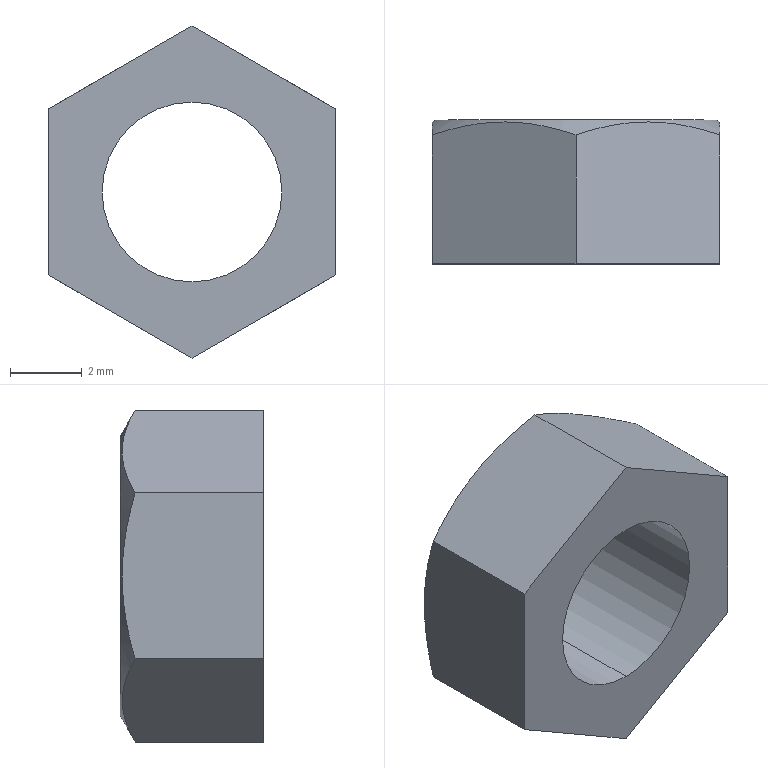Part | STEP file | NN19-M5 | 1 solid | 12 faces | box 8 x 4 x 9.238 mm | volume 142.232 mm3 | plane 8 | cylinder 2 | cone 2 | commonest cylinder face diameters 5 x2
STEP:
#1=CARTESIAN_POINT('',(0.,0.,0.));
#2=DIRECTION('',(0.,0.,1.));
#3=DIRECTION('',(1.,0.,0.));
#4=AXIS2_PLACEMENT_3D('',#1,#2,#3);
#5=CARTESIAN_POINT('',(0.,4.,-2.5));
#6=VERTEX_POINT('',#5);
#7=CARTESIAN_POINT('',(0.,0.,-2.5));
#8=VERTEX_POINT('',#7);
#9=CARTESIAN_POINT('',(0.,4.,-2.5));
#10=DIRECTION('',(0.,-1.,0.));
#11=VECTOR('',#10,1.);
#12=LINE('',#9,#11);
#13=CARTESIAN_POINT('',(0.,4.,0.));
#14=DIRECTION('',(0.,-1.,0.));
#15=DIRECTION('',(0.,0.,-1.));
#16=AXIS2_PLACEMENT_3D('',#13,#14,#15);
#17=CYLINDRICAL_SURFACE('',#16,2.5);
#18=CARTESIAN_POINT('',(6.283,0.));
#19=DIRECTION('',(0.,1.));
#20=VECTOR('',#19,1.);
#21=LINE('',#18,#20);
#22=(GEOMETRIC_REPRESENTATION_CONTEXT(2)PARAMETRIC_REPRESENTATION_CONTEXT()REPRESENTATION_CONTEXT('',''));
#23=DEFINITIONAL_REPRESENTATION('',(#21),#22);
#24=PCURVE('',#17,#23);
#25=CARTESIAN_POINT('',(0.,4.,0.));
#26=DIRECTION('',(0.,-1.,0.));
#27=DIRECTION('',(0.,0.,-1.));
#28=AXIS2_PLACEMENT_3D('',#25,#26,#27);
#29=CYLINDRICAL_SURFACE('',#28,2.5);
#30=CARTESIAN_POINT('',(0.,0.));
#31=DIRECTION('',(0.,1.));
#32=VECTOR('',#31,1.);
#33=LINE('',#30,#32);
#34=(GEOMETRIC_REPRESENTATION_CONTEXT(2)PARAMETRIC_REPRESENTATION_CONTEXT()REPRESENTATION_CONTEXT('',''));
#35=DEFINITIONAL_REPRESENTATION('',(#33),#34);
#36=PCURVE('',#29,#35);
#37=SURFACE_CURVE('',#12,(#24,#36),.PCURVE_S1.);
#38=EDGE_CURVE('',#6,#8,#37,.T.);
#39=ORIENTED_EDGE('',*,*,#38,.T.);
#40=CARTESIAN_POINT('',(0.,0.,2.5));
#41=VERTEX_POINT('',#40);
#42=CARTESIAN_POINT('',(0.,0.,0.));
#43=DIRECTION('',(0.,1.,0.));
#44=DIRECTION('',(0.,0.,1.));
#45=AXIS2_PLACEMENT_3D('',#42,#43,#44);
#46=CIRCLE('',#45,2.5);
#47=CARTESIAN_POINT('',(9.425,4.));
#48=DIRECTION('',(-1.,0.));
#49=VECTOR('',#48,1.);
#50=LINE('',#47,#49);
#51=(GEOMETRIC_REPRESENTATION_CONTEXT(2)PARAMETRIC_REPRESENTATION_CONTEXT()REPRESENTATION_CONTEXT('',''));
#52=DEFINITIONAL_REPRESENTATION('',(#50),#51);
#53=PCURVE('',#17,#52);
#54=CARTESIAN_POINT('',(0.,0.,0.));
#55=DIRECTION('',(0.,-1.,0.));
#56=DIRECTION('',(0.,0.,1.));
#57=AXIS2_PLACEMENT_3D('',#54,#55,#56);
#58=PLANE('',#57);
#59=CARTESIAN_POINT('',(2.5,0.));
#60=CARTESIAN_POINT('',(2.5,-4.33));
#61=CARTESIAN_POINT('',(-1.25,-2.165));
#62=CARTESIAN_POINT('',(-5.,0.));
#63=CARTESIAN_POINT('',(-1.25,2.165));
#64=CARTESIAN_POINT('',(2.5,4.33));
#65=CARTESIAN_POINT('',(2.5,0.));
#66=(BOUNDED_CURVE()B_SPLINE_CURVE(2,(#59,#60,#61,#62,#63,#64,#65),.UNSPECIFIED.,.T.,.F.)B_SPLINE_CURVE_WITH_KNOTS((1,2,2,2,2,1),(-2.094,0.,2.094,4.189,6.283,8.378),.UNSPECIFIED.)CURVE()GEOMETRIC_REPRESENTATION_ITEM()RATIONAL_B_SPLINE_CURVE((1.,0.5,1.,0.5,1.,0.5,1.))REPRESENTATION_ITEM(''));
#67=(GEOMETRIC_REPRESENTATION_CONTEXT(2)PARAMETRIC_REPRESENTATION_CONTEXT()REPRESENTATION_CONTEXT('',''));
#68=DEFINITIONAL_REPRESENTATION('',(#66),#67);
#69=PCURVE('',#58,#68);
#70=SURFACE_CURVE('',#46,(#53,#69),.PCURVE_S1.);
#71=EDGE_CURVE('',#8,#41,#70,.T.);
#72=ORIENTED_EDGE('',*,*,#71,.T.);
#73=CARTESIAN_POINT('',(0.,4.,2.5));
#74=VERTEX_POINT('',#73);
#75=CARTESIAN_POINT('',(0.,4.,2.5));
#76=DIRECTION('',(0.,-1.,0.));
#77=VECTOR('',#76,1.);
#78=LINE('',#75,#77);
#79=CARTESIAN_POINT('',(3.142,0.));
#80=DIRECTION('',(0.,1.));
#81=VECTOR('',#80,1.);
#82=LINE('',#79,#81);
#83=(GEOMETRIC_REPRESENTATION_CONTEXT(2)PARAMETRIC_REPRESENTATION_CONTEXT()REPRESENTATION_CONTEXT('',''));
#84=DEFINITIONAL_REPRESENTATION('',(#82),#83);
#85=PCURVE('',#17,#84);
#86=CARTESIAN_POINT('',(3.142,0.));
#87=DIRECTION('',(0.,1.));
#88=VECTOR('',#87,1.);
#89=LINE('',#86,#88);
#90=(GEOMETRIC_REPRESENTATION_CONTEXT(2)PARAMETRIC_REPRESENTATION_CONTEXT()REPRESENTATION_CONTEXT('',''));
#91=DEFINITIONAL_REPRESENTATION('',(#89),#90);
#92=PCURVE('',#29,#91);
#93=SURFACE_CURVE('',#78,(#85,#92),.PCURVE_S1.);
#94=EDGE_CURVE('',#74,#41,#93,.T.);
#95=ORIENTED_EDGE('',*,*,#94,.F.);
#96=CARTESIAN_POINT('',(0.,4.,0.));
#97=DIRECTION('',(0.,-1.,0.));
#98=DIRECTION('',(0.,0.,-1.));
#99=AXIS2_PLACEMENT_3D('',#96,#97,#98);
#100=CIRCLE('',#99,2.5);
#101=CARTESIAN_POINT('',(0.,0.));
#102=DIRECTION('',(1.,0.));
#103=VECTOR('',#102,1.);
#104=LINE('',#101,#103);
#105=(GEOMETRIC_REPRESENTATION_CONTEXT(2)PARAMETRIC_REPRESENTATION_CONTEXT()REPRESENTATION_CONTEXT('',''));
#106=DEFINITIONAL_REPRESENTATION('',(#104),#105);
#107=PCURVE('',#17,#106);
#108=CARTESIAN_POINT('',(0.,4.,0.));
#109=DIRECTION('',(0.,1.,0.));
#110=DIRECTION('',(-1.,0.,0.));
#111=AXIS2_PLACEMENT_3D('',#108,#109,#110);
#112=PLANE('',#111);
#113=CARTESIAN_POINT('',(0.,-2.5));
#114=CARTESIAN_POINT('',(-4.33,-2.5));
#115=CARTESIAN_POINT('',(-2.165,1.25));
#116=CARTESIAN_POINT('',(0.,5.));
#117=CARTESIAN_POINT('',(2.165,1.25));
#118=CARTESIAN_POINT('',(4.33,-2.5));
#119=CARTESIAN_POINT('',(0.,-2.5));
#120=(BOUNDED_CURVE()B_SPLINE_CURVE(2,(#113,#114,#115,#116,#117,#118,#119),.UNSPECIFIED.,.T.,.F.)B_SPLINE_CURVE_WITH_KNOTS((1,2,2,2,2,1),(-2.094,0.,2.094,4.189,6.283,8.378),.UNSPECIFIED.)CURVE()GEOMETRIC_REPRESENTATION_ITEM()RATIONAL_B_SPLINE_CURVE((1.,0.5,1.,0.5,1.,0.5,1.))REPRESENTATION_ITEM(''));
#121=(GEOMETRIC_REPRESENTATION_CONTEXT(2)PARAMETRIC_REPRESENTATION_CONTEXT()REPRESENTATION_CONTEXT('',''));
#122=DEFINITIONAL_REPRESENTATION('',(#120),#121);
#123=PCURVE('',#112,#122);
#124=SURFACE_CURVE('',#100,(#107,#123),.PCURVE_S1.);
#125=EDGE_CURVE('',#74,#6,#124,.T.);
#126=ORIENTED_EDGE('',*,*,#125,.T.);
#127=EDGE_LOOP('',(#39,#72,#95,#126));
#128=FACE_BOUND('',#127,.F.);
#129=ADVANCED_FACE('',(#128),#17,.F.);
#130=CARTESIAN_POINT('',(3.9,4.,0.));
#131=VERTEX_POINT('',#130);
#132=CARTESIAN_POINT('',(-3.9,4.,0.));
#133=VERTEX_POINT('',#132);
#134=CARTESIAN_POINT('',(0.,4.,0.));
#135=DIRECTION('',(0.,-1.,0.));
#136=DIRECTION('',(1.,0.,0.));
#137=AXIS2_PLACEMENT_3D('',#134,#135,#136);
#138=CIRCLE('',#137,3.9);
#139=CARTESIAN_POINT('',(0.,4.,0.));
#140=DIRECTION('',(0.,-1.,0.));
#141=DIRECTION('',(1.,0.,0.));
#142=AXIS2_PLACEMENT_3D('',#139,#140,#141);
#143=CONICAL_SURFACE('',#142,3.9,1.047);
#144=CARTESIAN_POINT('',(0.,0.));
#145=DIRECTION('',(1.,0.));
#146=VECTOR('',#145,1.);
#147=LINE('',#144,#146);
#148=(GEOMETRIC_REPRESENTATION_CONTEXT(2)PARAMETRIC_REPRESENTATION_CONTEXT()REPRESENTATION_CONTEXT('',''));
#149=DEFINITIONAL_REPRESENTATION('',(#147),#148);
#150=PCURVE('',#143,#149);
#151=CARTESIAN_POINT('',(-3.9,0.));
#152=CARTESIAN_POINT('',(-3.9,6.755));
#153=CARTESIAN_POINT('',(1.95,3.377));
#154=CARTESIAN_POINT('',(7.8,0.));
#155=CARTESIAN_POINT('',(1.95,-3.377));
#156=CARTESIAN_POINT('',(-3.9,-6.755));
#157=CARTESIAN_POINT('',(-3.9,0.));
#158=(BOUNDED_CURVE()B_SPLINE_CURVE(2,(#151,#152,#153,#154,#155,#156,#157),.UNSPECIFIED.,.T.,.F.)B_SPLINE_CURVE_WITH_KNOTS((1,2,2,2,2,1),(-2.094,0.,2.094,4.189,6.283,8.378),.UNSPECIFIED.)CURVE()GEOMETRIC_REPRESENTATION_ITEM()RATIONAL_B_SPLINE_CURVE((1.,0.5,1.,0.5,1.,0.5,1.))REPRESENTATION_ITEM(''));
#159=(GEOMETRIC_REPRESENTATION_CONTEXT(2)PARAMETRIC_REPRESENTATION_CONTEXT()REPRESENTATION_CONTEXT('',''));
#160=DEFINITIONAL_REPRESENTATION('',(#158),#159);
#161=PCURVE('',#112,#160);
#162=SURFACE_CURVE('',#138,(#150,#161),.PCURVE_S1.);
#163=EDGE_CURVE('',#131,#133,#162,.T.);
#164=ORIENTED_EDGE('',*,*,#163,.T.);
#165=CARTESIAN_POINT('',(-4.,3.942,0.));
#166=VERTEX_POINT('',#165);
#167=CARTESIAN_POINT('',(-3.9,4.,0.));
#168=DIRECTION('',(-0.866,-0.5,0.));
#169=VECTOR('',#168,1.);
#170=LINE('',#167,#169);
#171=CARTESIAN_POINT('',(3.142,0.));
#172=DIRECTION('',(0.,1.));
#173=VECTOR('',#172,1.);
#174=LINE('',#171,#173);
#175=(GEOMETRIC_REPRESENTATION_CONTEXT(2)PARAMETRIC_REPRESENTATION_CONTEXT()REPRESENTATION_CONTEXT('',''));
#176=DEFINITIONAL_REPRESENTATION('',(#174),#175);
#177=PCURVE('',#143,#176);
#178=CARTESIAN_POINT('',(0.,4.,0.));
#179=DIRECTION('',(0.,-1.,0.));
#180=DIRECTION('',(1.,0.,0.));
#181=AXIS2_PLACEMENT_3D('',#178,#179,#180);
#182=CONICAL_SURFACE('',#181,3.9,1.047);
#183=CARTESIAN_POINT('',(3.142,0.));
#184=DIRECTION('',(0.,1.));
#185=VECTOR('',#184,1.);
#186=LINE('',#183,#185);
#187=(GEOMETRIC_REPRESENTATION_CONTEXT(2)PARAMETRIC_REPRESENTATION_CONTEXT()REPRESENTATION_CONTEXT('',''));
#188=DEFINITIONAL_REPRESENTATION('',(#186),#187);
#189=PCURVE('',#182,#188);
#190=SURFACE_CURVE('',#170,(#177,#189),.PCURVE_S1.);
#191=EDGE_CURVE('',#133,#166,#190,.T.);
#192=ORIENTED_EDGE('',*,*,#191,.T.);
#193=CARTESIAN_POINT('',(-4.,3.585,2.309));
#194=VERTEX_POINT('',#193);
#195=CARTESIAN_POINT('',(-4.,3.585,2.309));
#196=CARTESIAN_POINT('',(-4.,3.802,1.557));
#197=CARTESIAN_POINT('',(-4.,3.942,0.7909));
#198=CARTESIAN_POINT('',(-4.,3.942,0.));
#199=B_SPLINE_CURVE_WITH_KNOTS('',3,(#195,#196,#197,#198),.UNSPECIFIED.,.F.,.F.,(4,4),(0.005037,0.007387),.PIECEWISE_BEZIER_KNOTS.);
#200=CARTESIAN_POINT('',(2.618,0.415));
#201=CARTESIAN_POINT('',(2.624,0.4051));
#202=CARTESIAN_POINT('',(2.637,0.3857));
#203=CARTESIAN_POINT('',(2.657,0.3575));
#204=CARTESIAN_POINT('',(2.678,0.3304));
#205=CARTESIAN_POINT('',(2.699,0.3043));
#206=CARTESIAN_POINT('',(2.72,0.2793));
#207=CARTESIAN_POINT('',(2.742,0.2554));
#208=CARTESIAN_POINT('',(2.764,0.2327));
#209=CARTESIAN_POINT('',(2.787,0.2112));
#210=CARTESIAN_POINT('',(2.81,0.1909));
#211=CARTESIAN_POINT('',(2.833,0.1719));
#212=CARTESIAN_POINT('',(2.857,0.1543));
#213=CARTESIAN_POINT('',(2.882,0.138));
#214=CARTESIAN_POINT('',(2.906,0.1231));
#215=CARTESIAN_POINT('',(2.931,0.1096));
#216=CARTESIAN_POINT('',(2.957,0.09762));
#217=CARTESIAN_POINT('',(2.982,0.08713));
#218=CARTESIAN_POINT('',(3.008,0.07817));
#219=CARTESIAN_POINT('',(3.035,0.07078));
#220=CARTESIAN_POINT('',(3.061,0.06499));
#221=CARTESIAN_POINT('',(3.088,0.06082));
#222=CARTESIAN_POINT('',(3.115,0.0583));
#223=CARTESIAN_POINT('',(3.133,0.05773));
#224=CARTESIAN_POINT('',(3.142,0.05774));
#225=B_SPLINE_CURVE_WITH_KNOTS('',3,(#200,#201,#202,#203,#204,#205,#206,#207,#208,#209,#210,#211,#212,#213,#214,#215,#216,#217,#218,#219,#220,#221,#222,#223,#224),.UNSPECIFIED.,.F.,.F.,(4,1,1,1,1,1,1,1,1,1,1,1,1,1,1,1,1,1,1,1,1,1,4),(0.005037,0.005144,0.005251,0.005357,0.005464,0.005571,0.005678,0.005785,0.005891,0.005998,0.006105,0.006212,0.006319,0.006425,0.006532,0.006639,0.006746,0.006853,0.006959,0.007066,0.007173,0.00728,0.007387),.QUASI_UNIFORM_KNOTS.);
#226=(GEOMETRIC_REPRESENTATION_CONTEXT(2)PARAMETRIC_REPRESENTATION_CONTEXT()REPRESENTATION_CONTEXT('',''));
#227=DEFINITIONAL_REPRESENTATION('',(#225),#226);
#228=PCURVE('',#143,#227);
#229=CARTESIAN_POINT('',(-4.,3.585,2.309));
#230=DIRECTION('',(1.,0.,0.));
#231=DIRECTION('',(0.,0.,1.));
#232=AXIS2_PLACEMENT_3D('',#229,#230,#231);
#233=PLANE('',#232);
#234=CARTESIAN_POINT('',(0.,0.));
#235=CARTESIAN_POINT('',(-0.7524,-0.2172));
#236=CARTESIAN_POINT('',(-1.518,-0.3573));
#237=CARTESIAN_POINT('',(-2.309,-0.3573));
#238=B_SPLINE_CURVE_WITH_KNOTS('',3,(#234,#235,#236,#237),.UNSPECIFIED.,.F.,.F.,(4,4),(0.005037,0.007387),.PIECEWISE_BEZIER_KNOTS.);
#239=(GEOMETRIC_REPRESENTATION_CONTEXT(2)PARAMETRIC_REPRESENTATION_CONTEXT()REPRESENTATION_CONTEXT('',''));
#240=DEFINITIONAL_REPRESENTATION('',(#238),#239);
#241=PCURVE('',#233,#240);
#242=SURFACE_CURVE('',#199,(#228,#241),.PCURVE_S1.);
#243=EDGE_CURVE('',#194,#166,#242,.T.);
#244=ORIENTED_EDGE('',*,*,#243,.F.);
#245=CARTESIAN_POINT('',(0.,3.585,4.619));
#246=VERTEX_POINT('',#245);
#247=CARTESIAN_POINT('',(0.,3.585,4.619));
#248=CARTESIAN_POINT('',(-0.6531,3.803,4.242));
#249=CARTESIAN_POINT('',(-1.316,3.942,3.859));
#250=CARTESIAN_POINT('',(-2.336,3.943,3.27));
#251=CARTESIAN_POINT('',(-2.676,3.908,3.074));
#252=CARTESIAN_POINT('',(-3.343,3.784,2.689));
#253=CARTESIAN_POINT('',(-3.673,3.694,2.498));
#254=CARTESIAN_POINT('',(-4.,3.585,2.309));
#255=B_SPLINE_CURVE_WITH_KNOTS('',3,(#247,#248,#249,#250,#251,#252,#253,#254),.UNSPECIFIED.,.F.,.F.,(4,2,2,4),(0.000000238,0.002333,0.003499,0.004665),.UNSPECIFIED.);
#256=CARTESIAN_POINT('',(1.571,0.415));
#257=CARTESIAN_POINT('',(1.584,0.3952));
#258=CARTESIAN_POINT('',(1.61,0.3569));
#259=CARTESIAN_POINT('',(1.651,0.3036));
#260=CARTESIAN_POINT('',(1.694,0.2546));
#261=CARTESIAN_POINT('',(1.739,0.2104));
#262=CARTESIAN_POINT('',(1.786,0.1712));
#263=CARTESIAN_POINT('',(1.834,0.1372));
#264=CARTESIAN_POINT('',(1.884,0.1089));
#265=CARTESIAN_POINT('',(1.935,0.08646));
#266=CARTESIAN_POINT('',(1.987,0.07011));
#267=CARTESIAN_POINT('',(2.04,0.0601));
#268=CARTESIAN_POINT('',(2.093,0.05662));
#269=CARTESIAN_POINT('',(2.147,0.05983));
#270=CARTESIAN_POINT('',(2.2,0.06961));
#271=CARTESIAN_POINT('',(2.252,0.08582));
#272=CARTESIAN_POINT('',(2.304,0.1082));
#273=CARTESIAN_POINT('',(2.354,0.1366));
#274=CARTESIAN_POINT('',(2.402,0.1706));
#275=CARTESIAN_POINT('',(2.449,0.2099));
#276=CARTESIAN_POINT('',(2.494,0.2543));
#277=CARTESIAN_POINT('',(2.537,0.3034));
#278=CARTESIAN_POINT('',(2.579,0.3568));
#279=CARTESIAN_POINT('',(2.605,0.3952));
#280=CARTESIAN_POINT('',(2.618,0.415));
#281=B_SPLINE_CURVE_WITH_KNOTS('',3,(#256,#257,#258,#259,#260,#261,#262,#263,#264,#265,#266,#267,#268,#269,#270,#271,#272,#273,#274,#275,#276,#277,#278,#279,#280),.UNSPECIFIED.,.F.,.F.,(4,1,1,1,1,1,1,1,1,1,1,1,1,1,1,1,1,1,1,1,1,1,4),(0.000000238,0.0002123,0.0004243,0.0006363,0.0008484,0.00106,0.001272,0.001484,0.001697,0.001909,0.002121,0.002333,0.002545,0.002757,0.002969,0.003181,0.003393,0.003605,0.003817,0.004029,0.004241,0.004453,0.004665),.QUASI_UNIFORM_KNOTS.);
#282=(GEOMETRIC_REPRESENTATION_CONTEXT(2)PARAMETRIC_REPRESENTATION_CONTEXT()REPRESENTATION_CONTEXT('',''));
#283=DEFINITIONAL_REPRESENTATION('',(#281),#282);
#284=PCURVE('',#143,#283);
#285=CARTESIAN_POINT('',(0.,3.585,4.619));
#286=DIRECTION('',(0.5,0.,-0.866));
#287=DIRECTION('',(0.866,0.,0.5));
#288=AXIS2_PLACEMENT_3D('',#285,#286,#287);
#289=PLANE('',#288);
#290=CARTESIAN_POINT('',(0.,0.));
#291=CARTESIAN_POINT('',(-0.7542,-0.2177));
#292=CARTESIAN_POINT('',(-1.52,-0.3568));
#293=CARTESIAN_POINT('',(-2.698,-0.3575));
#294=CARTESIAN_POINT('',(-3.09,-0.3234));
#295=CARTESIAN_POINT('',(-3.861,-0.1989));
#296=CARTESIAN_POINT('',(-4.241,-0.109));
#297=CARTESIAN_POINT('',(-4.619,0.));
#298=B_SPLINE_CURVE_WITH_KNOTS('',3,(#290,#291,#292,#293,#294,#295,#296,#297),.UNSPECIFIED.,.F.,.F.,(4,2,2,4),(0.000000238,0.002333,0.003499,0.004665),.UNSPECIFIED.);
#299=(GEOMETRIC_REPRESENTATION_CONTEXT(2)PARAMETRIC_REPRESENTATION_CONTEXT()REPRESENTATION_CONTEXT('',''));
#300=DEFINITIONAL_REPRESENTATION('',(#298),#299);
#301=PCURVE('',#289,#300);
#302=SURFACE_CURVE('',#255,(#284,#301),.PCURVE_S1.);
#303=EDGE_CURVE('',#246,#194,#302,.T.);
#304=ORIENTED_EDGE('',*,*,#303,.F.);
#305=CARTESIAN_POINT('',(4.,3.585,2.309));
#306=VERTEX_POINT('',#305);
#307=CARTESIAN_POINT('',(4.,3.585,2.309));
#308=CARTESIAN_POINT('',(3.347,3.803,2.686));
#309=CARTESIAN_POINT('',(2.684,3.942,3.069));
#310=CARTESIAN_POINT('',(1.664,3.943,3.658));
#311=CARTESIAN_POINT('',(1.324,3.908,3.854));
#312=CARTESIAN_POINT('',(0.6567,3.784,4.24));
#313=CARTESIAN_POINT('',(0.327,3.694,4.43));
#314=CARTESIAN_POINT('',(0.,3.585,4.619));
#315=B_SPLINE_CURVE_WITH_KNOTS('',3,(#307,#308,#309,#310,#311,#312,#313,#314),.UNSPECIFIED.,.F.,.F.,(4,2,2,4),(0.000000238,0.002333,0.003499,0.004665),.UNSPECIFIED.);
#316=CARTESIAN_POINT('',(0.5236,0.415));
#317=CARTESIAN_POINT('',(0.5365,0.3952));
#318=CARTESIAN_POINT('',(0.5628,0.3569));
#319=CARTESIAN_POINT('',(0.6041,0.3036));
#320=CARTESIAN_POINT('',(0.6472,0.2546));
#321=CARTESIAN_POINT('',(0.6921,0.2104));
#322=CARTESIAN_POINT('',(0.7388,0.1712));
#323=CARTESIAN_POINT('',(0.787,0.1372));
#324=CARTESIAN_POINT('',(0.8367,0.1089));
#325=CARTESIAN_POINT('',(0.8877,0.08646));
#326=CARTESIAN_POINT('',(0.9398,0.07011));
#327=CARTESIAN_POINT('',(0.9926,0.0601));
#328=CARTESIAN_POINT('',(1.046,0.05662));
#329=CARTESIAN_POINT('',(1.1,0.05983));
#330=CARTESIAN_POINT('',(1.153,0.06961));
#331=CARTESIAN_POINT('',(1.205,0.08582));
#332=CARTESIAN_POINT('',(1.257,0.1082));
#333=CARTESIAN_POINT('',(1.307,0.1366));
#334=CARTESIAN_POINT('',(1.355,0.1706));
#335=CARTESIAN_POINT('',(1.402,0.2099));
#336=CARTESIAN_POINT('',(1.447,0.2543));
#337=CARTESIAN_POINT('',(1.49,0.3034));
#338=CARTESIAN_POINT('',(1.532,0.3568));
#339=CARTESIAN_POINT('',(1.558,0.3952));
#340=CARTESIAN_POINT('',(1.571,0.415));
#341=B_SPLINE_CURVE_WITH_KNOTS('',3,(#316,#317,#318,#319,#320,#321,#322,#323,#324,#325,#326,#327,#328,#329,#330,#331,#332,#333,#334,#335,#336,#337,#338,#339,#340),.UNSPECIFIED.,.F.,.F.,(4,1,1,1,1,1,1,1,1,1,1,1,1,1,1,1,1,1,1,1,1,1,4),(0.000000238,0.0002123,0.0004243,0.0006363,0.0008484,0.00106,0.001272,0.001484,0.001697,0.001909,0.002121,0.002333,0.002545,0.002757,0.002969,0.003181,0.003393,0.003605,0.003817,0.004029,0.004241,0.004453,0.004665),.QUASI_UNIFORM_KNOTS.);
#342=(GEOMETRIC_REPRESENTATION_CONTEXT(2)PARAMETRIC_REPRESENTATION_CONTEXT()REPRESENTATION_CONTEXT('',''));
#343=DEFINITIONAL_REPRESENTATION('',(#341),#342);
#344=PCURVE('',#143,#343);
#345=CARTESIAN_POINT('',(4.,3.585,2.309));
#346=DIRECTION('',(-0.5,0.,-0.866));
#347=DIRECTION('',(0.866,0.,-0.5));
#348=AXIS2_PLACEMENT_3D('',#345,#346,#347);
#349=PLANE('',#348);
#350=CARTESIAN_POINT('',(0.,0.));
#351=CARTESIAN_POINT('',(-0.7542,-0.2177));
#352=CARTESIAN_POINT('',(-1.52,-0.3568));
#353=CARTESIAN_POINT('',(-2.698,-0.3575));
#354=CARTESIAN_POINT('',(-3.09,-0.3234));
#355=CARTESIAN_POINT('',(-3.861,-0.1989));
#356=CARTESIAN_POINT('',(-4.241,-0.109));
#357=CARTESIAN_POINT('',(-4.619,0.));
#358=B_SPLINE_CURVE_WITH_KNOTS('',3,(#350,#351,#352,#353,#354,#355,#356,#357),.UNSPECIFIED.,.F.,.F.,(4,2,2,4),(0.000000238,0.002333,0.003499,0.004665),.UNSPECIFIED.);
#359=(GEOMETRIC_REPRESENTATION_CONTEXT(2)PARAMETRIC_REPRESENTATION_CONTEXT()REPRESENTATION_CONTEXT('',''));
#360=DEFINITIONAL_REPRESENTATION('',(#358),#359);
#361=PCURVE('',#349,#360);
#362=SURFACE_CURVE('',#315,(#344,#361),.PCURVE_S1.);
#363=EDGE_CURVE('',#306,#246,#362,.T.);
#364=ORIENTED_EDGE('',*,*,#363,.F.);
#365=CARTESIAN_POINT('',(4.,3.942,0.));
#366=VERTEX_POINT('',#365);
#367=CARTESIAN_POINT('',(4.,3.942,0.));
#368=CARTESIAN_POINT('',(4.,3.942,0.7905));
#369=CARTESIAN_POINT('',(4.,3.802,1.558));
#370=CARTESIAN_POINT('',(4.,3.585,2.309));
#371=B_SPLINE_CURVE_WITH_KNOTS('',3,(#367,#368,#369,#370),.UNSPECIFIED.,.F.,.F.,(4,4),(0.007387,0.009735),.PIECEWISE_BEZIER_KNOTS.);
#372=CARTESIAN_POINT('',(0.,0.05774));
#373=CARTESIAN_POINT('',(0.008983,0.05773));
#374=CARTESIAN_POINT('',(0.02693,0.0583));
#375=CARTESIAN_POINT('',(0.05373,0.06082));
#376=CARTESIAN_POINT('',(0.08039,0.06499));
#377=CARTESIAN_POINT('',(0.1069,0.07078));
#378=CARTESIAN_POINT('',(0.1331,0.07817));
#379=CARTESIAN_POINT('',(0.1591,0.08714));
#380=CARTESIAN_POINT('',(0.1849,0.09763));
#381=CARTESIAN_POINT('',(0.2103,0.1096));
#382=CARTESIAN_POINT('',(0.2354,0.1231));
#383=CARTESIAN_POINT('',(0.2601,0.138));
#384=CARTESIAN_POINT('',(0.2845,0.1543));
#385=CARTESIAN_POINT('',(0.3084,0.172));
#386=CARTESIAN_POINT('',(0.332,0.191));
#387=CARTESIAN_POINT('',(0.3551,0.2112));
#388=CARTESIAN_POINT('',(0.3778,0.2328));
#389=CARTESIAN_POINT('',(0.4,0.2555));
#390=CARTESIAN_POINT('',(0.4218,0.2793));
#391=CARTESIAN_POINT('',(0.4431,0.3044));
#392=CARTESIAN_POINT('',(0.4639,0.3304));
#393=CARTESIAN_POINT('',(0.4843,0.3576));
#394=CARTESIAN_POINT('',(0.5042,0.3857));
#395=CARTESIAN_POINT('',(0.5172,0.4051));
#396=CARTESIAN_POINT('',(0.5236,0.415));
#397=B_SPLINE_CURVE_WITH_KNOTS('',3,(#372,#373,#374,#375,#376,#377,#378,#379,#380,#381,#382,#383,#384,#385,#386,#387,#388,#389,#390,#391,#392,#393,#394,#395,#396),.UNSPECIFIED.,.F.,.F.,(4,1,1,1,1,1,1,1,1,1,1,1,1,1,1,1,1,1,1,1,1,1,4),(0.007387,0.007493,0.0076,0.007707,0.007814,0.00792,0.008027,0.008134,0.00824,0.008347,0.008454,0.008561,0.008667,0.008774,0.008881,0.008988,0.009094,0.009201,0.009308,0.009415,0.009521,0.009628,0.009735),.QUASI_UNIFORM_KNOTS.);
#398=(GEOMETRIC_REPRESENTATION_CONTEXT(2)PARAMETRIC_REPRESENTATION_CONTEXT()REPRESENTATION_CONTEXT('',''));
#399=DEFINITIONAL_REPRESENTATION('',(#397),#398);
#400=PCURVE('',#143,#399);
#401=CARTESIAN_POINT('',(4.,3.585,-2.309));
#402=DIRECTION('',(-1.,0.,0.));
#403=DIRECTION('',(0.,0.,-1.));
#404=AXIS2_PLACEMENT_3D('',#401,#402,#403);
#405=PLANE('',#404);
#406=CARTESIAN_POINT('',(-2.309,-0.3573));
#407=CARTESIAN_POINT('',(-3.1,-0.3573));
#408=CARTESIAN_POINT('',(-3.867,-0.2169));
#409=CARTESIAN_POINT('',(-4.619,0.));
#410=B_SPLINE_CURVE_WITH_KNOTS('',3,(#406,#407,#408,#409),.UNSPECIFIED.,.F.,.F.,(4,4),(0.007387,0.009735),.PIECEWISE_BEZIER_KNOTS.);
#411=(GEOMETRIC_REPRESENTATION_CONTEXT(2)PARAMETRIC_REPRESENTATION_CONTEXT()REPRESENTATION_CONTEXT('',''));
#412=DEFINITIONAL_REPRESENTATION('',(#410),#411);
#413=PCURVE('',#405,#412);
#414=SURFACE_CURVE('',#371,(#400,#413),.PCURVE_S1.);
#415=EDGE_CURVE('',#366,#306,#414,.T.);
#416=ORIENTED_EDGE('',*,*,#415,.F.);
#417=CARTESIAN_POINT('',(3.9,4.,0.));
#418=DIRECTION('',(0.866,-0.5,0.));
#419=VECTOR('',#418,1.);
#420=LINE('',#417,#419);
#421=CARTESIAN_POINT('',(0.,0.));
#422=DIRECTION('',(0.,1.));
#423=VECTOR('',#422,1.);
#424=LINE('',#421,#423);
#425=(GEOMETRIC_REPRESENTATION_CONTEXT(2)PARAMETRIC_REPRESENTATION_CONTEXT()REPRESENTATION_CONTEXT('',''));
#426=DEFINITIONAL_REPRESENTATION('',(#424),#425);
#427=PCURVE('',#143,#426);
#428=CARTESIAN_POINT('',(6.283,0.));
#429=DIRECTION('',(0.,1.));
#430=VECTOR('',#429,1.);
#431=LINE('',#428,#430);
#432=(GEOMETRIC_REPRESENTATION_CONTEXT(2)PARAMETRIC_REPRESENTATION_CONTEXT()REPRESENTATION_CONTEXT('',''));
#433=DEFINITIONAL_REPRESENTATION('',(#431),#432);
#434=PCURVE('',#182,#433);
#435=SURFACE_CURVE('',#420,(#427,#434),.PCURVE_S1.);
#436=EDGE_CURVE('',#131,#366,#435,.T.);
#437=ORIENTED_EDGE('',*,*,#436,.F.);
#438=EDGE_LOOP('',(#164,#192,#244,#304,#364,#416,#437));
#439=FACE_BOUND('',#438,.T.);
#440=ADVANCED_FACE('',(#439),#143,.T.);
#441=ORIENTED_EDGE('',*,*,#191,.F.);
#442=CARTESIAN_POINT('',(0.,4.,0.));
#443=DIRECTION('',(0.,-1.,0.));
#444=DIRECTION('',(1.,0.,0.));
#445=AXIS2_PLACEMENT_3D('',#442,#443,#444);
#446=CIRCLE('',#445,3.9);
#447=CARTESIAN_POINT('',(0.,0.));
#448=DIRECTION('',(1.,0.));
#449=VECTOR('',#448,1.);
#450=LINE('',#447,#449);
#451=(GEOMETRIC_REPRESENTATION_CONTEXT(2)PARAMETRIC_REPRESENTATION_CONTEXT()REPRESENTATION_CONTEXT('',''));
#452=DEFINITIONAL_REPRESENTATION('',(#450),#451);
#453=PCURVE('',#182,#452);
#454=CARTESIAN_POINT('',(-3.9,0.));
#455=CARTESIAN_POINT('',(-3.9,6.755));
#456=CARTESIAN_POINT('',(1.95,3.377));
#457=CARTESIAN_POINT('',(7.8,0.));
#458=CARTESIAN_POINT('',(1.95,-3.377));
#459=CARTESIAN_POINT('',(-3.9,-6.755));
#460=CARTESIAN_POINT('',(-3.9,0.));
#461=(BOUNDED_CURVE()B_SPLINE_CURVE(2,(#454,#455,#456,#457,#458,#459,#460),.UNSPECIFIED.,.T.,.F.)B_SPLINE_CURVE_WITH_KNOTS((1,2,2,2,2,1),(-2.094,0.,2.094,4.189,6.283,8.378),.UNSPECIFIED.)CURVE()GEOMETRIC_REPRESENTATION_ITEM()RATIONAL_B_SPLINE_CURVE((1.,0.5,1.,0.5,1.,0.5,1.))REPRESENTATION_ITEM(''));
#462=(GEOMETRIC_REPRESENTATION_CONTEXT(2)PARAMETRIC_REPRESENTATION_CONTEXT()REPRESENTATION_CONTEXT('',''));
#463=DEFINITIONAL_REPRESENTATION('',(#461),#462);
#464=PCURVE('',#112,#463);
#465=SURFACE_CURVE('',#446,(#453,#464),.PCURVE_S1.);
#466=EDGE_CURVE('',#133,#131,#465,.T.);
#467=ORIENTED_EDGE('',*,*,#466,.T.);
#468=ORIENTED_EDGE('',*,*,#436,.T.);
#469=CARTESIAN_POINT('',(4.,3.585,-2.309));
#470=VERTEX_POINT('',#469);
#471=CARTESIAN_POINT('',(4.,3.585,-2.309));
#472=CARTESIAN_POINT('',(4.,3.802,-1.557));
#473=CARTESIAN_POINT('',(4.,3.942,-0.7909));
#474=CARTESIAN_POINT('',(4.,3.942,0.));
#475=B_SPLINE_CURVE_WITH_KNOTS('',3,(#471,#472,#473,#474),.UNSPECIFIED.,.F.,.F.,(4,4),(0.005037,0.007387),.PIECEWISE_BEZIER_KNOTS.);
#476=CARTESIAN_POINT('',(5.76,0.415));
#477=CARTESIAN_POINT('',(5.766,0.4051));
#478=CARTESIAN_POINT('',(5.779,0.3857));
#479=CARTESIAN_POINT('',(5.799,0.3575));
#480=CARTESIAN_POINT('',(5.819,0.3304));
#481=CARTESIAN_POINT('',(5.84,0.3043));
#482=CARTESIAN_POINT('',(5.861,0.2793));
#483=CARTESIAN_POINT('',(5.883,0.2554));
#484=CARTESIAN_POINT('',(5.905,0.2327));
#485=CARTESIAN_POINT('',(5.928,0.2112));
#486=CARTESIAN_POINT('',(5.951,0.1909));
#487=CARTESIAN_POINT('',(5.975,0.1719));
#488=CARTESIAN_POINT('',(5.999,0.1543));
#489=CARTESIAN_POINT('',(6.023,0.138));
#490=CARTESIAN_POINT('',(6.048,0.1231));
#491=CARTESIAN_POINT('',(6.073,0.1096));
#492=CARTESIAN_POINT('',(6.098,0.09762));
#493=CARTESIAN_POINT('',(6.124,0.08713));
#494=CARTESIAN_POINT('',(6.15,0.07817));
#495=CARTESIAN_POINT('',(6.176,0.07078));
#496=CARTESIAN_POINT('',(6.203,0.06499));
#497=CARTESIAN_POINT('',(6.229,0.06082));
#498=CARTESIAN_POINT('',(6.256,0.0583));
#499=CARTESIAN_POINT('',(6.274,0.05773));
#500=CARTESIAN_POINT('',(6.283,0.05774));
#501=B_SPLINE_CURVE_WITH_KNOTS('',3,(#476,#477,#478,#479,#480,#481,#482,#483,#484,#485,#486,#487,#488,#489,#490,#491,#492,#493,#494,#495,#496,#497,#498,#499,#500),.UNSPECIFIED.,.F.,.F.,(4,1,1,1,1,1,1,1,1,1,1,1,1,1,1,1,1,1,1,1,1,1,4),(0.005037,0.005144,0.005251,0.005357,0.005464,0.005571,0.005678,0.005785,0.005891,0.005998,0.006105,0.006212,0.006319,0.006425,0.006532,0.006639,0.006746,0.006853,0.006959,0.007066,0.007173,0.00728,0.007387),.QUASI_UNIFORM_KNOTS.);
#502=(GEOMETRIC_REPRESENTATION_CONTEXT(2)PARAMETRIC_REPRESENTATION_CONTEXT()REPRESENTATION_CONTEXT('',''));
#503=DEFINITIONAL_REPRESENTATION('',(#501),#502);
#504=PCURVE('',#182,#503);
#505=CARTESIAN_POINT('',(0.,0.));
#506=CARTESIAN_POINT('',(-0.7524,-0.2172));
#507=CARTESIAN_POINT('',(-1.518,-0.3573));
#508=CARTESIAN_POINT('',(-2.309,-0.3573));
#509=B_SPLINE_CURVE_WITH_KNOTS('',3,(#505,#506,#507,#508),.UNSPECIFIED.,.F.,.F.,(4,4),(0.005037,0.007387),.PIECEWISE_BEZIER_KNOTS.);
#510=(GEOMETRIC_REPRESENTATION_CONTEXT(2)PARAMETRIC_REPRESENTATION_CONTEXT()REPRESENTATION_CONTEXT('',''));
#511=DEFINITIONAL_REPRESENTATION('',(#509),#510);
#512=PCURVE('',#405,#511);
#513=SURFACE_CURVE('',#475,(#504,#512),.PCURVE_S1.);
#514=EDGE_CURVE('',#470,#366,#513,.T.);
#515=ORIENTED_EDGE('',*,*,#514,.F.);
#516=CARTESIAN_POINT('',(0.,3.585,-4.619));
#517=VERTEX_POINT('',#516);
#518=CARTESIAN_POINT('',(0.,3.585,-4.619));
#519=CARTESIAN_POINT('',(0.6531,3.803,-4.242));
#520=CARTESIAN_POINT('',(1.316,3.942,-3.859));
#521=CARTESIAN_POINT('',(2.336,3.943,-3.27));
#522=CARTESIAN_POINT('',(2.676,3.908,-3.074));
#523=CARTESIAN_POINT('',(3.343,3.784,-2.689));
#524=CARTESIAN_POINT('',(3.673,3.694,-2.498));
#525=CARTESIAN_POINT('',(4.,3.585,-2.309));
#526=B_SPLINE_CURVE_WITH_KNOTS('',3,(#518,#519,#520,#521,#522,#523,#524,#525),.UNSPECIFIED.,.F.,.F.,(4,2,2,4),(0.000000238,0.002333,0.003499,0.004665),.UNSPECIFIED.);
#527=CARTESIAN_POINT('',(4.712,0.415));
#528=CARTESIAN_POINT('',(4.725,0.3952));
#529=CARTESIAN_POINT('',(4.752,0.3569));
#530=CARTESIAN_POINT('',(4.793,0.3036));
#531=CARTESIAN_POINT('',(4.836,0.2546));
#532=CARTESIAN_POINT('',(4.881,0.2104));
#533=CARTESIAN_POINT('',(4.928,0.1712));
#534=CARTESIAN_POINT('',(4.976,0.1372));
#535=CARTESIAN_POINT('',(5.026,0.1089));
#536=CARTESIAN_POINT('',(5.076,0.08646));
#537=CARTESIAN_POINT('',(5.129,0.07011));
#538=CARTESIAN_POINT('',(5.181,0.0601));
#539=CARTESIAN_POINT('',(5.235,0.05662));
#540=CARTESIAN_POINT('',(5.288,0.05983));
#541=CARTESIAN_POINT('',(5.342,0.06961));
#542=CARTESIAN_POINT('',(5.394,0.08582));
#543=CARTESIAN_POINT('',(5.445,0.1082));
#544=CARTESIAN_POINT('',(5.495,0.1366));
#545=CARTESIAN_POINT('',(5.544,0.1706));
#546=CARTESIAN_POINT('',(5.591,0.2099));
#547=CARTESIAN_POINT('',(5.636,0.2543));
#548=CARTESIAN_POINT('',(5.679,0.3034));
#549=CARTESIAN_POINT('',(5.72,0.3568));
#550=CARTESIAN_POINT('',(5.747,0.3952));
#551=CARTESIAN_POINT('',(5.76,0.415));
#552=B_SPLINE_CURVE_WITH_KNOTS('',3,(#527,#528,#529,#530,#531,#532,#533,#534,#535,#536,#537,#538,#539,#540,#541,#542,#543,#544,#545,#546,#547,#548,#549,#550,#551),.UNSPECIFIED.,.F.,.F.,(4,1,1,1,1,1,1,1,1,1,1,1,1,1,1,1,1,1,1,1,1,1,4),(0.000000238,0.0002123,0.0004243,0.0006363,0.0008484,0.00106,0.001272,0.001484,0.001697,0.001909,0.002121,0.002333,0.002545,0.002757,0.002969,0.003181,0.003393,0.003605,0.003817,0.004029,0.004241,0.004453,0.004665),.QUASI_UNIFORM_KNOTS.);
#553=(GEOMETRIC_REPRESENTATION_CONTEXT(2)PARAMETRIC_REPRESENTATION_CONTEXT()REPRESENTATION_CONTEXT('',''));
#554=DEFINITIONAL_REPRESENTATION('',(#552),#553);
#555=PCURVE('',#182,#554);
#556=CARTESIAN_POINT('',(0.,3.585,-4.619));
#557=DIRECTION('',(-0.5,0.,0.866));
#558=DIRECTION('',(-0.866,0.,-0.5));
#559=AXIS2_PLACEMENT_3D('',#556,#557,#558);
#560=PLANE('',#559);
#561=CARTESIAN_POINT('',(0.,0.));
#562=CARTESIAN_POINT('',(-0.7542,-0.2177));
#563=CARTESIAN_POINT('',(-1.52,-0.3568));
#564=CARTESIAN_POINT('',(-2.698,-0.3575));
#565=CARTESIAN_POINT('',(-3.09,-0.3234));
#566=CARTESIAN_POINT('',(-3.861,-0.1989));
#567=CARTESIAN_POINT('',(-4.241,-0.109));
#568=CARTESIAN_POINT('',(-4.619,0.));
#569=B_SPLINE_CURVE_WITH_KNOTS('',3,(#561,#562,#563,#564,#565,#566,#567,#568),.UNSPECIFIED.,.F.,.F.,(4,2,2,4),(0.000000238,0.002333,0.003499,0.004665),.UNSPECIFIED.);
#570=(GEOMETRIC_REPRESENTATION_CONTEXT(2)PARAMETRIC_REPRESENTATION_CONTEXT()REPRESENTATION_CONTEXT('',''));
#571=DEFINITIONAL_REPRESENTATION('',(#569),#570);
#572=PCURVE('',#560,#571);
#573=SURFACE_CURVE('',#526,(#555,#572),.PCURVE_S1.);
#574=EDGE_CURVE('',#517,#470,#573,.T.);
#575=ORIENTED_EDGE('',*,*,#574,.F.);
#576=CARTESIAN_POINT('',(-4.,3.585,-2.309));
#577=VERTEX_POINT('',#576);
#578=CARTESIAN_POINT('',(-4.,3.585,-2.309));
#579=CARTESIAN_POINT('',(-3.347,3.803,-2.686));
#580=CARTESIAN_POINT('',(-2.684,3.942,-3.069));
#581=CARTESIAN_POINT('',(-1.664,3.943,-3.658));
#582=CARTESIAN_POINT('',(-1.324,3.908,-3.854));
#583=CARTESIAN_POINT('',(-0.6567,3.784,-4.24));
#584=CARTESIAN_POINT('',(-0.327,3.694,-4.43));
#585=CARTESIAN_POINT('',(0.,3.585,-4.619));
#586=B_SPLINE_CURVE_WITH_KNOTS('',3,(#578,#579,#580,#581,#582,#583,#584,#585),.UNSPECIFIED.,.F.,.F.,(4,2,2,4),(0.000000238,0.002333,0.003499,0.004665),.UNSPECIFIED.);
#587=CARTESIAN_POINT('',(3.665,0.415));
#588=CARTESIAN_POINT('',(3.678,0.3952));
#589=CARTESIAN_POINT('',(3.704,0.3569));
#590=CARTESIAN_POINT('',(3.746,0.3036));
#591=CARTESIAN_POINT('',(3.789,0.2546));
#592=CARTESIAN_POINT('',(3.834,0.2104));
#593=CARTESIAN_POINT('',(3.88,0.1712));
#594=CARTESIAN_POINT('',(3.929,0.1372));
#595=CARTESIAN_POINT('',(3.978,0.1089));
#596=CARTESIAN_POINT('',(4.029,0.08646));
#597=CARTESIAN_POINT('',(4.081,0.07011));
#598=CARTESIAN_POINT('',(4.134,0.0601));
#599=CARTESIAN_POINT('',(4.188,0.05662));
#600=CARTESIAN_POINT('',(4.241,0.05983));
#601=CARTESIAN_POINT('',(4.294,0.06961));
#602=CARTESIAN_POINT('',(4.347,0.08582));
#603=CARTESIAN_POINT('',(4.398,0.1082));
#604=CARTESIAN_POINT('',(4.448,0.1366));
#605=CARTESIAN_POINT('',(4.497,0.1706));
#606=CARTESIAN_POINT('',(4.543,0.2099));
#607=CARTESIAN_POINT('',(4.589,0.2543));
#608=CARTESIAN_POINT('',(4.632,0.3034));
#609=CARTESIAN_POINT('',(4.673,0.3568));
#610=CARTESIAN_POINT('',(4.7,0.3952));
#611=CARTESIAN_POINT('',(4.712,0.415));
#612=B_SPLINE_CURVE_WITH_KNOTS('',3,(#587,#588,#589,#590,#591,#592,#593,#594,#595,#596,#597,#598,#599,#600,#601,#602,#603,#604,#605,#606,#607,#608,#609,#610,#611),.UNSPECIFIED.,.F.,.F.,(4,1,1,1,1,1,1,1,1,1,1,1,1,1,1,1,1,1,1,1,1,1,4),(0.000000238,0.0002123,0.0004243,0.0006363,0.0008484,0.00106,0.001272,0.001484,0.001697,0.001909,0.002121,0.002333,0.002545,0.002757,0.002969,0.003181,0.003393,0.003605,0.003817,0.004029,0.004241,0.004453,0.004665),.QUASI_UNIFORM_KNOTS.);
#613=(GEOMETRIC_REPRESENTATION_CONTEXT(2)PARAMETRIC_REPRESENTATION_CONTEXT()REPRESENTATION_CONTEXT('',''));
#614=DEFINITIONAL_REPRESENTATION('',(#612),#613);
#615=PCURVE('',#182,#614);
#616=CARTESIAN_POINT('',(-4.,3.585,-2.309));
#617=DIRECTION('',(0.5,0.,0.866));
#618=DIRECTION('',(-0.866,0.,0.5));
#619=AXIS2_PLACEMENT_3D('',#616,#617,#618);
#620=PLANE('',#619);
#621=CARTESIAN_POINT('',(0.,0.));
#622=CARTESIAN_POINT('',(-0.7542,-0.2177));
#623=CARTESIAN_POINT('',(-1.52,-0.3568));
#624=CARTESIAN_POINT('',(-2.698,-0.3575));
#625=CARTESIAN_POINT('',(-3.09,-0.3234));
#626=CARTESIAN_POINT('',(-3.861,-0.1989));
#627=CARTESIAN_POINT('',(-4.241,-0.109));
#628=CARTESIAN_POINT('',(-4.619,0.));
#629=B_SPLINE_CURVE_WITH_KNOTS('',3,(#621,#622,#623,#624,#625,#626,#627,#628),.UNSPECIFIED.,.F.,.F.,(4,2,2,4),(0.000000238,0.002333,0.003499,0.004665),.UNSPECIFIED.);
#630=(GEOMETRIC_REPRESENTATION_CONTEXT(2)PARAMETRIC_REPRESENTATION_CONTEXT()REPRESENTATION_CONTEXT('',''));
#631=DEFINITIONAL_REPRESENTATION('',(#629),#630);
#632=PCURVE('',#620,#631);
#633=SURFACE_CURVE('',#586,(#615,#632),.PCURVE_S1.);
#634=EDGE_CURVE('',#577,#517,#633,.T.);
#635=ORIENTED_EDGE('',*,*,#634,.F.);
#636=CARTESIAN_POINT('',(-4.,3.942,0.));
#637=CARTESIAN_POINT('',(-4.,3.942,-0.7905));
#638=CARTESIAN_POINT('',(-4.,3.802,-1.558));
#639=CARTESIAN_POINT('',(-4.,3.585,-2.309));
#640=B_SPLINE_CURVE_WITH_KNOTS('',3,(#636,#637,#638,#639),.UNSPECIFIED.,.F.,.F.,(4,4),(0.007387,0.009735),.PIECEWISE_BEZIER_KNOTS.);
#641=CARTESIAN_POINT('',(3.142,0.05774));
#642=CARTESIAN_POINT('',(3.151,0.05773));
#643=CARTESIAN_POINT('',(3.169,0.0583));
#644=CARTESIAN_POINT('',(3.195,0.06082));
#645=CARTESIAN_POINT('',(3.222,0.06499));
#646=CARTESIAN_POINT('',(3.248,0.07078));
#647=CARTESIAN_POINT('',(3.275,0.07817));
#648=CARTESIAN_POINT('',(3.301,0.08714));
#649=CARTESIAN_POINT('',(3.326,0.09763));
#650=CARTESIAN_POINT('',(3.352,0.1096));
#651=CARTESIAN_POINT('',(3.377,0.1231));
#652=CARTESIAN_POINT('',(3.402,0.138));
#653=CARTESIAN_POINT('',(3.426,0.1543));
#654=CARTESIAN_POINT('',(3.45,0.172));
#655=CARTESIAN_POINT('',(3.474,0.191));
#656=CARTESIAN_POINT('',(3.497,0.2112));
#657=CARTESIAN_POINT('',(3.519,0.2328));
#658=CARTESIAN_POINT('',(3.542,0.2555));
#659=CARTESIAN_POINT('',(3.563,0.2793));
#660=CARTESIAN_POINT('',(3.585,0.3044));
#661=CARTESIAN_POINT('',(3.606,0.3304));
#662=CARTESIAN_POINT('',(3.626,0.3576));
#663=CARTESIAN_POINT('',(3.646,0.3857));
#664=CARTESIAN_POINT('',(3.659,0.4051));
#665=CARTESIAN_POINT('',(3.665,0.415));
#666=B_SPLINE_CURVE_WITH_KNOTS('',3,(#641,#642,#643,#644,#645,#646,#647,#648,#649,#650,#651,#652,#653,#654,#655,#656,#657,#658,#659,#660,#661,#662,#663,#664,#665),.UNSPECIFIED.,.F.,.F.,(4,1,1,1,1,1,1,1,1,1,1,1,1,1,1,1,1,1,1,1,1,1,4),(0.007387,0.007493,0.0076,0.007707,0.007814,0.00792,0.008027,0.008134,0.00824,0.008347,0.008454,0.008561,0.008667,0.008774,0.008881,0.008988,0.009094,0.009201,0.009308,0.009415,0.009521,0.009628,0.009735),.QUASI_UNIFORM_KNOTS.);
#667=(GEOMETRIC_REPRESENTATION_CONTEXT(2)PARAMETRIC_REPRESENTATION_CONTEXT()REPRESENTATION_CONTEXT('',''));
#668=DEFINITIONAL_REPRESENTATION('',(#666),#667);
#669=PCURVE('',#182,#668);
#670=CARTESIAN_POINT('',(-2.309,-0.3573));
#671=CARTESIAN_POINT('',(-3.1,-0.3573));
#672=CARTESIAN_POINT('',(-3.867,-0.2169));
#673=CARTESIAN_POINT('',(-4.619,0.));
#674=B_SPLINE_CURVE_WITH_KNOTS('',3,(#670,#671,#672,#673),.UNSPECIFIED.,.F.,.F.,(4,4),(0.007387,0.009735),.PIECEWISE_BEZIER_KNOTS.);
#675=(GEOMETRIC_REPRESENTATION_CONTEXT(2)PARAMETRIC_REPRESENTATION_CONTEXT()REPRESENTATION_CONTEXT('',''));
#676=DEFINITIONAL_REPRESENTATION('',(#674),#675);
#677=PCURVE('',#233,#676);
#678=SURFACE_CURVE('',#640,(#669,#677),.PCURVE_S1.);
#679=EDGE_CURVE('',#166,#577,#678,.T.);
#680=ORIENTED_EDGE('',*,*,#679,.F.);
#681=EDGE_LOOP('',(#441,#467,#468,#515,#575,#635,#680));
#682=FACE_BOUND('',#681,.T.);
#683=ADVANCED_FACE('',(#682),#182,.T.);
#684=CARTESIAN_POINT('',(0.,4.,0.));
#685=DIRECTION('',(0.,-1.,0.));
#686=DIRECTION('',(0.,0.,-1.));
#687=AXIS2_PLACEMENT_3D('',#684,#685,#686);
#688=CIRCLE('',#687,2.5);
#689=CARTESIAN_POINT('',(0.,-2.5));
#690=CARTESIAN_POINT('',(-4.33,-2.5));
#691=CARTESIAN_POINT('',(-2.165,1.25));
#692=CARTESIAN_POINT('',(0.,5.));
#693=CARTESIAN_POINT('',(2.165,1.25));
#694=CARTESIAN_POINT('',(4.33,-2.5));
#695=CARTESIAN_POINT('',(0.,-2.5));
#696=(BOUNDED_CURVE()B_SPLINE_CURVE(2,(#689,#690,#691,#692,#693,#694,#695),.UNSPECIFIED.,.T.,.F.)B_SPLINE_CURVE_WITH_KNOTS((1,2,2,2,2,1),(-2.094,0.,2.094,4.189,6.283,8.378),.UNSPECIFIED.)CURVE()GEOMETRIC_REPRESENTATION_ITEM()RATIONAL_B_SPLINE_CURVE((1.,0.5,1.,0.5,1.,0.5,1.))REPRESENTATION_ITEM(''));
#697=(GEOMETRIC_REPRESENTATION_CONTEXT(2)PARAMETRIC_REPRESENTATION_CONTEXT()REPRESENTATION_CONTEXT('',''));
#698=DEFINITIONAL_REPRESENTATION('',(#696),#697);
#699=PCURVE('',#112,#698);
#700=CARTESIAN_POINT('',(0.,0.));
#701=DIRECTION('',(1.,0.));
#702=VECTOR('',#701,1.);
#703=LINE('',#700,#702);
#704=(GEOMETRIC_REPRESENTATION_CONTEXT(2)PARAMETRIC_REPRESENTATION_CONTEXT()REPRESENTATION_CONTEXT('',''));
#705=DEFINITIONAL_REPRESENTATION('',(#703),#704);
#706=PCURVE('',#29,#705);
#707=SURFACE_CURVE('',#688,(#699,#706),.PCURVE_S1.);
#708=EDGE_CURVE('',#6,#74,#707,.T.);
#709=ORIENTED_EDGE('',*,*,#708,.T.);
#710=ORIENTED_EDGE('',*,*,#125,.T.);
#711=EDGE_LOOP('',(#709,#710));
#712=FACE_BOUND('',#711,.T.);
#713=ORIENTED_EDGE('',*,*,#163,.F.);
#714=ORIENTED_EDGE('',*,*,#466,.F.);
#715=EDGE_LOOP('',(#713,#714));
#716=FACE_BOUND('',#715,.T.);
#717=ADVANCED_FACE('',(#712,#716),#112,.T.);
#718=ORIENTED_EDGE('',*,*,#514,.T.);
#719=ORIENTED_EDGE('',*,*,#415,.T.);
#720=CARTESIAN_POINT('',(4.,0.,2.309));
#721=VERTEX_POINT('',#720);
#722=CARTESIAN_POINT('',(4.,0.,2.309));
#723=DIRECTION('',(0.,1.,0.));
#724=VECTOR('',#723,1.);
#725=LINE('',#722,#724);
#726=CARTESIAN_POINT('',(-4.619,3.585));
#727=DIRECTION('',(0.,-1.));
#728=VECTOR('',#727,1.);
#729=LINE('',#726,#728);
#730=(GEOMETRIC_REPRESENTATION_CONTEXT(2)PARAMETRIC_REPRESENTATION_CONTEXT()REPRESENTATION_CONTEXT('',''));
#731=DEFINITIONAL_REPRESENTATION('',(#729),#730);
#732=PCURVE('',#405,#731);
#733=CARTESIAN_POINT('',(0.,3.585));
#734=DIRECTION('',(0.,-1.));
#735=VECTOR('',#734,1.);
#736=LINE('',#733,#735);
#737=(GEOMETRIC_REPRESENTATION_CONTEXT(2)PARAMETRIC_REPRESENTATION_CONTEXT()REPRESENTATION_CONTEXT('',''));
#738=DEFINITIONAL_REPRESENTATION('',(#736),#737);
#739=PCURVE('',#349,#738);
#740=SURFACE_CURVE('',#725,(#732,#739),.PCURVE_S1.);
#741=EDGE_CURVE('',#721,#306,#740,.T.);
#742=ORIENTED_EDGE('',*,*,#741,.F.);
#743=CARTESIAN_POINT('',(4.,0.,-2.309));
#744=VERTEX_POINT('',#743);
#745=CARTESIAN_POINT('',(4.,0.,-2.309));
#746=DIRECTION('',(0.,0.,1.));
#747=VECTOR('',#746,1.);
#748=LINE('',#745,#747);
#749=CARTESIAN_POINT('',(0.,3.585));
#750=DIRECTION('',(-1.,0.));
#751=VECTOR('',#750,1.);
#752=LINE('',#749,#751);
#753=(GEOMETRIC_REPRESENTATION_CONTEXT(2)PARAMETRIC_REPRESENTATION_CONTEXT()REPRESENTATION_CONTEXT('',''));
#754=DEFINITIONAL_REPRESENTATION('',(#752),#753);
#755=PCURVE('',#405,#754);
#756=CARTESIAN_POINT('',(-2.309,-4.));
#757=DIRECTION('',(1.,0.));
#758=VECTOR('',#757,1.);
#759=LINE('',#756,#758);
#760=(GEOMETRIC_REPRESENTATION_CONTEXT(2)PARAMETRIC_REPRESENTATION_CONTEXT()REPRESENTATION_CONTEXT('',''));
#761=DEFINITIONAL_REPRESENTATION('',(#759),#760);
#762=PCURVE('',#58,#761);
#763=SURFACE_CURVE('',#748,(#755,#762),.PCURVE_S1.);
#764=EDGE_CURVE('',#744,#721,#763,.T.);
#765=ORIENTED_EDGE('',*,*,#764,.F.);
#766=CARTESIAN_POINT('',(4.,0.,-2.309));
#767=DIRECTION('',(0.,1.,0.));
#768=VECTOR('',#767,1.);
#769=LINE('',#766,#768);
#770=CARTESIAN_POINT('',(0.,3.585));
#771=DIRECTION('',(0.,-1.));
#772=VECTOR('',#771,1.);
#773=LINE('',#770,#772);
#774=(GEOMETRIC_REPRESENTATION_CONTEXT(2)PARAMETRIC_REPRESENTATION_CONTEXT()REPRESENTATION_CONTEXT('',''));
#775=DEFINITIONAL_REPRESENTATION('',(#773),#774);
#776=PCURVE('',#405,#775);
#777=CARTESIAN_POINT('',(-4.619,3.585));
#778=DIRECTION('',(0.,-1.));
#779=VECTOR('',#778,1.);
#780=LINE('',#777,#779);
#781=(GEOMETRIC_REPRESENTATION_CONTEXT(2)PARAMETRIC_REPRESENTATION_CONTEXT()REPRESENTATION_CONTEXT('',''));
#782=DEFINITIONAL_REPRESENTATION('',(#780),#781);
#783=PCURVE('',#560,#782);
#784=SURFACE_CURVE('',#769,(#776,#783),.PCURVE_S1.);
#785=EDGE_CURVE('',#744,#470,#784,.T.);
#786=ORIENTED_EDGE('',*,*,#785,.T.);
#787=EDGE_LOOP('',(#718,#719,#742,#765,#786));
#788=FACE_BOUND('',#787,.T.);
#789=ADVANCED_FACE('',(#788),#405,.F.);
#790=ORIENTED_EDGE('',*,*,#574,.T.);
#791=ORIENTED_EDGE('',*,*,#785,.F.);
#792=CARTESIAN_POINT('',(0.,0.,-4.619));
#793=VERTEX_POINT('',#792);
#794=CARTESIAN_POINT('',(0.,0.,-4.619));
#795=DIRECTION('',(0.866,0.,0.5));
#796=VECTOR('',#795,1.);
#797=LINE('',#794,#796);
#798=CARTESIAN_POINT('',(0.,3.585));
#799=DIRECTION('',(-1.,0.));
#800=VECTOR('',#799,1.);
#801=LINE('',#798,#800);
#802=(GEOMETRIC_REPRESENTATION_CONTEXT(2)PARAMETRIC_REPRESENTATION_CONTEXT()REPRESENTATION_CONTEXT('',''));
#803=DEFINITIONAL_REPRESENTATION('',(#801),#802);
#804=PCURVE('',#560,#803);
#805=CARTESIAN_POINT('',(-4.619,0.));
#806=DIRECTION('',(0.5,-0.866));
#807=VECTOR('',#806,1.);
#808=LINE('',#805,#807);
#809=(GEOMETRIC_REPRESENTATION_CONTEXT(2)PARAMETRIC_REPRESENTATION_CONTEXT()REPRESENTATION_CONTEXT('',''));
#810=DEFINITIONAL_REPRESENTATION('',(#808),#809);
#811=PCURVE('',#58,#810);
#812=SURFACE_CURVE('',#797,(#804,#811),.PCURVE_S1.);
#813=EDGE_CURVE('',#793,#744,#812,.T.);
#814=ORIENTED_EDGE('',*,*,#813,.F.);
#815=CARTESIAN_POINT('',(0.,0.,-4.619));
#816=DIRECTION('',(0.,1.,0.));
#817=VECTOR('',#816,1.);
#818=LINE('',#815,#817);
#819=CARTESIAN_POINT('',(0.,3.585));
#820=DIRECTION('',(0.,-1.));
#821=VECTOR('',#820,1.);
#822=LINE('',#819,#821);
#823=(GEOMETRIC_REPRESENTATION_CONTEXT(2)PARAMETRIC_REPRESENTATION_CONTEXT()REPRESENTATION_CONTEXT('',''));
#824=DEFINITIONAL_REPRESENTATION('',(#822),#823);
#825=PCURVE('',#560,#824);
#826=CARTESIAN_POINT('',(-4.619,3.585));
#827=DIRECTION('',(0.,-1.));
#828=VECTOR('',#827,1.);
#829=LINE('',#826,#828);
#830=(GEOMETRIC_REPRESENTATION_CONTEXT(2)PARAMETRIC_REPRESENTATION_CONTEXT()REPRESENTATION_CONTEXT('',''));
#831=DEFINITIONAL_REPRESENTATION('',(#829),#830);
#832=PCURVE('',#620,#831);
#833=SURFACE_CURVE('',#818,(#825,#832),.PCURVE_S1.);
#834=EDGE_CURVE('',#793,#517,#833,.T.);
#835=ORIENTED_EDGE('',*,*,#834,.T.);
#836=EDGE_LOOP('',(#790,#791,#814,#835));
#837=FACE_BOUND('',#836,.T.);
#838=ADVANCED_FACE('',(#837),#560,.F.);
#839=ORIENTED_EDGE('',*,*,#634,.T.);
#840=ORIENTED_EDGE('',*,*,#834,.F.);
#841=CARTESIAN_POINT('',(-4.,0.,-2.309));
#842=VERTEX_POINT('',#841);
#843=CARTESIAN_POINT('',(-4.,0.,-2.309));
#844=DIRECTION('',(0.866,0.,-0.5));
#845=VECTOR('',#844,1.);
#846=LINE('',#843,#845);
#847=CARTESIAN_POINT('',(0.,3.585));
#848=DIRECTION('',(-1.,0.));
#849=VECTOR('',#848,1.);
#850=LINE('',#847,#849);
#851=(GEOMETRIC_REPRESENTATION_CONTEXT(2)PARAMETRIC_REPRESENTATION_CONTEXT()REPRESENTATION_CONTEXT('',''));
#852=DEFINITIONAL_REPRESENTATION('',(#850),#851);
#853=PCURVE('',#620,#852);
#854=CARTESIAN_POINT('',(-2.309,4.));
#855=DIRECTION('',(-0.5,-0.866));
#856=VECTOR('',#855,1.);
#857=LINE('',#854,#856);
#858=(GEOMETRIC_REPRESENTATION_CONTEXT(2)PARAMETRIC_REPRESENTATION_CONTEXT()REPRESENTATION_CONTEXT('',''));
#859=DEFINITIONAL_REPRESENTATION('',(#857),#858);
#860=PCURVE('',#58,#859);
#861=SURFACE_CURVE('',#846,(#853,#860),.PCURVE_S1.);
#862=EDGE_CURVE('',#842,#793,#861,.T.);
#863=ORIENTED_EDGE('',*,*,#862,.F.);
#864=CARTESIAN_POINT('',(-4.,0.,-2.309));
#865=DIRECTION('',(0.,1.,0.));
#866=VECTOR('',#865,1.);
#867=LINE('',#864,#866);
#868=CARTESIAN_POINT('',(0.,3.585));
#869=DIRECTION('',(0.,-1.));
#870=VECTOR('',#869,1.);
#871=LINE('',#868,#870);
#872=(GEOMETRIC_REPRESENTATION_CONTEXT(2)PARAMETRIC_REPRESENTATION_CONTEXT()REPRESENTATION_CONTEXT('',''));
#873=DEFINITIONAL_REPRESENTATION('',(#871),#872);
#874=PCURVE('',#620,#873);
#875=CARTESIAN_POINT('',(-4.619,3.585));
#876=DIRECTION('',(0.,-1.));
#877=VECTOR('',#876,1.);
#878=LINE('',#875,#877);
#879=(GEOMETRIC_REPRESENTATION_CONTEXT(2)PARAMETRIC_REPRESENTATION_CONTEXT()REPRESENTATION_CONTEXT('',''));
#880=DEFINITIONAL_REPRESENTATION('',(#878),#879);
#881=PCURVE('',#233,#880);
#882=SURFACE_CURVE('',#867,(#874,#881),.PCURVE_S1.);
#883=EDGE_CURVE('',#842,#577,#882,.T.);
#884=ORIENTED_EDGE('',*,*,#883,.T.);
#885=EDGE_LOOP('',(#839,#840,#863,#884));
#886=FACE_BOUND('',#885,.T.);
#887=ADVANCED_FACE('',(#886),#620,.F.);
#888=ORIENTED_EDGE('',*,*,#243,.T.);
#889=ORIENTED_EDGE('',*,*,#679,.T.);
#890=ORIENTED_EDGE('',*,*,#883,.F.);
#891=CARTESIAN_POINT('',(-4.,0.,2.309));
#892=VERTEX_POINT('',#891);
#893=CARTESIAN_POINT('',(-4.,0.,2.309));
#894=DIRECTION('',(0.,0.,-1.));
#895=VECTOR('',#894,1.);
#896=LINE('',#893,#895);
#897=CARTESIAN_POINT('',(0.,3.585));
#898=DIRECTION('',(-1.,0.));
#899=VECTOR('',#898,1.);
#900=LINE('',#897,#899);
#901=(GEOMETRIC_REPRESENTATION_CONTEXT(2)PARAMETRIC_REPRESENTATION_CONTEXT()REPRESENTATION_CONTEXT('',''));
#902=DEFINITIONAL_REPRESENTATION('',(#900),#901);
#903=PCURVE('',#233,#902);
#904=CARTESIAN_POINT('',(2.309,4.));
#905=DIRECTION('',(-1.,0.));
#906=VECTOR('',#905,1.);
#907=LINE('',#904,#906);
#908=(GEOMETRIC_REPRESENTATION_CONTEXT(2)PARAMETRIC_REPRESENTATION_CONTEXT()REPRESENTATION_CONTEXT('',''));
#909=DEFINITIONAL_REPRESENTATION('',(#907),#908);
#910=PCURVE('',#58,#909);
#911=SURFACE_CURVE('',#896,(#903,#910),.PCURVE_S1.);
#912=EDGE_CURVE('',#892,#842,#911,.T.);
#913=ORIENTED_EDGE('',*,*,#912,.F.);
#914=CARTESIAN_POINT('',(-4.,0.,2.309));
#915=DIRECTION('',(0.,1.,0.));
#916=VECTOR('',#915,1.);
#917=LINE('',#914,#916);
#918=CARTESIAN_POINT('',(0.,3.585));
#919=DIRECTION('',(0.,-1.));
#920=VECTOR('',#919,1.);
#921=LINE('',#918,#920);
#922=(GEOMETRIC_REPRESENTATION_CONTEXT(2)PARAMETRIC_REPRESENTATION_CONTEXT()REPRESENTATION_CONTEXT('',''));
#923=DEFINITIONAL_REPRESENTATION('',(#921),#922);
#924=PCURVE('',#233,#923);
#925=CARTESIAN_POINT('',(-4.619,3.585));
#926=DIRECTION('',(0.,-1.));
#927=VECTOR('',#926,1.);
#928=LINE('',#925,#927);
#929=(GEOMETRIC_REPRESENTATION_CONTEXT(2)PARAMETRIC_REPRESENTATION_CONTEXT()REPRESENTATION_CONTEXT('',''));
#930=DEFINITIONAL_REPRESENTATION('',(#928),#929);
#931=PCURVE('',#289,#930);
#932=SURFACE_CURVE('',#917,(#924,#931),.PCURVE_S1.);
#933=EDGE_CURVE('',#892,#194,#932,.T.);
#934=ORIENTED_EDGE('',*,*,#933,.T.);
#935=EDGE_LOOP('',(#888,#889,#890,#913,#934));
#936=FACE_BOUND('',#935,.T.);
#937=ADVANCED_FACE('',(#936),#233,.F.);
#938=ORIENTED_EDGE('',*,*,#303,.T.);
#939=ORIENTED_EDGE('',*,*,#933,.F.);
#940=CARTESIAN_POINT('',(0.,0.,4.619));
#941=VERTEX_POINT('',#940);
#942=CARTESIAN_POINT('',(0.,0.,4.619));
#943=DIRECTION('',(-0.866,0.,-0.5));
#944=VECTOR('',#943,1.);
#945=LINE('',#942,#944);
#946=CARTESIAN_POINT('',(0.,3.585));
#947=DIRECTION('',(-1.,0.));
#948=VECTOR('',#947,1.);
#949=LINE('',#946,#948);
#950=(GEOMETRIC_REPRESENTATION_CONTEXT(2)PARAMETRIC_REPRESENTATION_CONTEXT()REPRESENTATION_CONTEXT('',''));
#951=DEFINITIONAL_REPRESENTATION('',(#949),#950);
#952=PCURVE('',#289,#951);
#953=CARTESIAN_POINT('',(4.619,0.));
#954=DIRECTION('',(-0.5,0.866));
#955=VECTOR('',#954,1.);
#956=LINE('',#953,#955);
#957=(GEOMETRIC_REPRESENTATION_CONTEXT(2)PARAMETRIC_REPRESENTATION_CONTEXT()REPRESENTATION_CONTEXT('',''));
#958=DEFINITIONAL_REPRESENTATION('',(#956),#957);
#959=PCURVE('',#58,#958);
#960=SURFACE_CURVE('',#945,(#952,#959),.PCURVE_S1.);
#961=EDGE_CURVE('',#941,#892,#960,.T.);
#962=ORIENTED_EDGE('',*,*,#961,.F.);
#963=CARTESIAN_POINT('',(0.,0.,4.619));
#964=DIRECTION('',(0.,1.,0.));
#965=VECTOR('',#964,1.);
#966=LINE('',#963,#965);
#967=CARTESIAN_POINT('',(0.,3.585));
#968=DIRECTION('',(0.,-1.));
#969=VECTOR('',#968,1.);
#970=LINE('',#967,#969);
#971=(GEOMETRIC_REPRESENTATION_CONTEXT(2)PARAMETRIC_REPRESENTATION_CONTEXT()REPRESENTATION_CONTEXT('',''));
#972=DEFINITIONAL_REPRESENTATION('',(#970),#971);
#973=PCURVE('',#289,#972);
#974=CARTESIAN_POINT('',(-4.619,3.585));
#975=DIRECTION('',(0.,-1.));
#976=VECTOR('',#975,1.);
#977=LINE('',#974,#976);
#978=(GEOMETRIC_REPRESENTATION_CONTEXT(2)PARAMETRIC_REPRESENTATION_CONTEXT()REPRESENTATION_CONTEXT('',''));
#979=DEFINITIONAL_REPRESENTATION('',(#977),#978);
#980=PCURVE('',#349,#979);
#981=SURFACE_CURVE('',#966,(#973,#980),.PCURVE_S1.);
#982=EDGE_CURVE('',#941,#246,#981,.T.);
#983=ORIENTED_EDGE('',*,*,#982,.T.);
#984=EDGE_LOOP('',(#938,#939,#962,#983));
#985=FACE_BOUND('',#984,.T.);
#986=ADVANCED_FACE('',(#985),#289,.F.);
#987=ORIENTED_EDGE('',*,*,#363,.T.);
#988=ORIENTED_EDGE('',*,*,#982,.F.);
#989=CARTESIAN_POINT('',(4.,0.,2.309));
#990=DIRECTION('',(-0.866,0.,0.5));
#991=VECTOR('',#990,1.);
#992=LINE('',#989,#991);
#993=CARTESIAN_POINT('',(0.,3.585));
#994=DIRECTION('',(-1.,0.));
#995=VECTOR('',#994,1.);
#996=LINE('',#993,#995);
#997=(GEOMETRIC_REPRESENTATION_CONTEXT(2)PARAMETRIC_REPRESENTATION_CONTEXT()REPRESENTATION_CONTEXT('',''));
#998=DEFINITIONAL_REPRESENTATION('',(#996),#997);
#999=PCURVE('',#349,#998);
#1000=CARTESIAN_POINT('',(2.309,-4.));
#1001=DIRECTION('',(0.5,0.866));
#1002=VECTOR('',#1001,1.);
#1003=LINE('',#1000,#1002);
#1004=(GEOMETRIC_REPRESENTATION_CONTEXT(2)PARAMETRIC_REPRESENTATION_CONTEXT()REPRESENTATION_CONTEXT('',''));
#1005=DEFINITIONAL_REPRESENTATION('',(#1003),#1004);
#1006=PCURVE('',#58,#1005);
#1007=SURFACE_CURVE('',#992,(#999,#1006),.PCURVE_S1.);
#1008=EDGE_CURVE('',#721,#941,#1007,.T.);
#1009=ORIENTED_EDGE('',*,*,#1008,.F.);
#1010=ORIENTED_EDGE('',*,*,#741,.T.);
#1011=EDGE_LOOP('',(#987,#988,#1009,#1010));
#1012=FACE_BOUND('',#1011,.T.);
#1013=ADVANCED_FACE('',(#1012),#349,.F.);
#1014=ORIENTED_EDGE('',*,*,#71,.T.);
#1015=CARTESIAN_POINT('',(0.,0.,0.));
#1016=DIRECTION('',(0.,1.,0.));
#1017=DIRECTION('',(0.,0.,1.));
#1018=AXIS2_PLACEMENT_3D('',#1015,#1016,#1017);
#1019=CIRCLE('',#1018,2.5);
#1020=CARTESIAN_POINT('',(2.5,0.));
#1021=CARTESIAN_POINT('',(2.5,-4.33));
#1022=CARTESIAN_POINT('',(-1.25,-2.165));
#1023=CARTESIAN_POINT('',(-5.,0.));
#1024=CARTESIAN_POINT('',(-1.25,2.165));
#1025=CARTESIAN_POINT('',(2.5,4.33));
#1026=CARTESIAN_POINT('',(2.5,0.));
#1027=(BOUNDED_CURVE()B_SPLINE_CURVE(2,(#1020,#1021,#1022,#1023,#1024,#1025,#1026),.UNSPECIFIED.,.T.,.F.)B_SPLINE_CURVE_WITH_KNOTS((1,2,2,2,2,1),(-2.094,0.,2.094,4.189,6.283,8.378),.UNSPECIFIED.)CURVE()GEOMETRIC_REPRESENTATION_ITEM()RATIONAL_B_SPLINE_CURVE((1.,0.5,1.,0.5,1.,0.5,1.))REPRESENTATION_ITEM(''));
#1028=(GEOMETRIC_REPRESENTATION_CONTEXT(2)PARAMETRIC_REPRESENTATION_CONTEXT()REPRESENTATION_CONTEXT('',''));
#1029=DEFINITIONAL_REPRESENTATION('',(#1027),#1028);
#1030=PCURVE('',#58,#1029);
#1031=CARTESIAN_POINT('',(3.142,4.));
#1032=DIRECTION('',(-1.,0.));
#1033=VECTOR('',#1032,1.);
#1034=LINE('',#1031,#1033);
#1035=(GEOMETRIC_REPRESENTATION_CONTEXT(2)PARAMETRIC_REPRESENTATION_CONTEXT()REPRESENTATION_CONTEXT('',''));
#1036=DEFINITIONAL_REPRESENTATION('',(#1034),#1035);
#1037=PCURVE('',#29,#1036);
#1038=SURFACE_CURVE('',#1019,(#1030,#1037),.PCURVE_S1.);
#1039=EDGE_CURVE('',#41,#8,#1038,.T.);
#1040=ORIENTED_EDGE('',*,*,#1039,.T.);
#1041=EDGE_LOOP('',(#1014,#1040));
#1042=FACE_BOUND('',#1041,.T.);
#1043=ORIENTED_EDGE('',*,*,#1008,.T.);
#1044=ORIENTED_EDGE('',*,*,#961,.T.);
#1045=ORIENTED_EDGE('',*,*,#912,.T.);
#1046=ORIENTED_EDGE('',*,*,#862,.T.);
#1047=ORIENTED_EDGE('',*,*,#813,.T.);
#1048=ORIENTED_EDGE('',*,*,#764,.T.);
#1049=EDGE_LOOP('',(#1043,#1044,#1045,#1046,#1047,#1048));
#1050=FACE_BOUND('',#1049,.T.);
#1051=ADVANCED_FACE('',(#1042,#1050),#58,.T.);
#1052=ORIENTED_EDGE('',*,*,#1039,.T.);
#1053=ORIENTED_EDGE('',*,*,#38,.F.);
#1054=ORIENTED_EDGE('',*,*,#708,.T.);
#1055=ORIENTED_EDGE('',*,*,#94,.T.);
#1056=EDGE_LOOP('',(#1052,#1053,#1054,#1055));
#1057=FACE_BOUND('',#1056,.F.);
#1058=ADVANCED_FACE('',(#1057),#29,.F.);
#1059=CLOSED_SHELL('',(#129,#440,#683,#717,#789,#838,#887,#937,#986,#1013,#1051,#1058));
#1060=MANIFOLD_SOLID_BREP('',#1059);
#1061=(LENGTH_UNIT()NAMED_UNIT(*)SI_UNIT(.MILLI.,.METRE.));
#1062=UNCERTAINTY_MEASURE_WITH_UNIT(LENGTH_MEASURE(0.0002),#1061,'','');
#1063=(NAMED_UNIT(*)PLANE_ANGLE_UNIT()SI_UNIT($,.RADIAN.));
#1064=(NAMED_UNIT(*)SI_UNIT($,.STERADIAN.)SOLID_ANGLE_UNIT());
#1065=(GEOMETRIC_REPRESENTATION_CONTEXT(3)GLOBAL_UNCERTAINTY_ASSIGNED_CONTEXT((#1062))GLOBAL_UNIT_ASSIGNED_CONTEXT((#1061,#1063,#1064))REPRESENTATION_CONTEXT('',''));
#1066=ADVANCED_BREP_SHAPE_REPRESENTATION('',(#4,#1060),#1065);